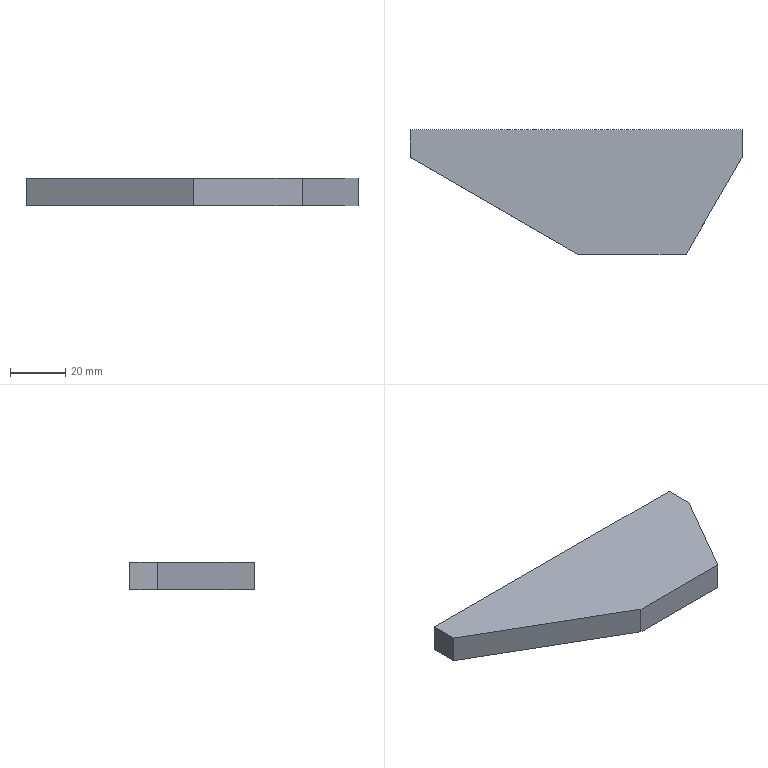Part | SolidWorks | features Extrusion 1 | 1 solid | 8 faces | box 120 x 45 x 10 mm | volume 39855 mm3 | plane 8
STEP:
#1=CARTESIAN_POINT('',(0.,0.,0.));
#2=VERTEX_POINT('',#1);
#3=CARTESIAN_POINT('',(0.,-10.,0.));
#4=VERTEX_POINT('',#3);
#5=CARTESIAN_POINT('',(0.,0.,0.));
#6=DIRECTION('',(0.,-1.,0.));
#7=VECTOR('',#6,1000.);
#8=LINE('',#5,#7);
#9=EDGE_CURVE('',#2,#4,#8,.T.);
#10=ORIENTED_EDGE('',*,*,#9,.T.);
#11=CARTESIAN_POINT('',(0.,-10.,10.));
#12=VERTEX_POINT('',#11);
#13=CARTESIAN_POINT('',(0.,-10.,10.));
#14=DIRECTION('',(0.,0.,-1.));
#15=VECTOR('',#14,1000.);
#16=LINE('',#13,#15);
#17=EDGE_CURVE('',#12,#4,#16,.T.);
#18=ORIENTED_EDGE('',*,*,#17,.F.);
#19=CARTESIAN_POINT('',(0.,0.,10.));
#20=VERTEX_POINT('',#19);
#21=CARTESIAN_POINT('',(0.,0.,10.));
#22=DIRECTION('',(0.,-1.,0.));
#23=VECTOR('',#22,1000.);
#24=LINE('',#21,#23);
#25=EDGE_CURVE('',#20,#12,#24,.T.);
#26=ORIENTED_EDGE('',*,*,#25,.F.);
#27=CARTESIAN_POINT('',(0.,0.,10.));
#28=DIRECTION('',(0.,0.,-1.));
#29=VECTOR('',#28,1000.);
#30=LINE('',#27,#29);
#31=EDGE_CURVE('',#20,#2,#30,.T.);
#32=ORIENTED_EDGE('',*,*,#31,.T.);
#33=EDGE_LOOP('',(#10,#18,#26,#32));
#34=FACE_OUTER_BOUND('',#33,.T.);
#35=CARTESIAN_POINT('',(0.,0.,10.));
#36=DIRECTION('',(1.,0.,0.));
#37=DIRECTION('',(0.,0.,-1.));
#38=AXIS2_PLACEMENT_3D('',#35,#36,#37);
#39=PLANE('',#38);
#40=ADVANCED_FACE('',(#34),#39,.F.);
#41=CARTESIAN_POINT('',(60.622,-45.,0.));
#42=VERTEX_POINT('',#41);
#43=CARTESIAN_POINT('',(60.622,-45.,0.));
#44=DIRECTION('',(0.866,-0.5,0.));
#45=VECTOR('',#44,1000.);
#46=LINE('',#43,#45);
#47=EDGE_CURVE('',#4,#42,#46,.T.);
#48=ORIENTED_EDGE('',*,*,#47,.T.);
#49=CARTESIAN_POINT('',(60.622,-45.,10.));
#50=VERTEX_POINT('',#49);
#51=CARTESIAN_POINT('',(60.622,-45.,10.));
#52=DIRECTION('',(0.,0.,-1.));
#53=VECTOR('',#52,1000.);
#54=LINE('',#51,#53);
#55=EDGE_CURVE('',#50,#42,#54,.T.);
#56=ORIENTED_EDGE('',*,*,#55,.F.);
#57=CARTESIAN_POINT('',(60.622,-45.,10.));
#58=DIRECTION('',(0.866,-0.5,0.));
#59=VECTOR('',#58,1000.);
#60=LINE('',#57,#59);
#61=EDGE_CURVE('',#12,#50,#60,.T.);
#62=ORIENTED_EDGE('',*,*,#61,.F.);
#63=ORIENTED_EDGE('',*,*,#17,.T.);
#64=EDGE_LOOP('',(#48,#56,#62,#63));
#65=FACE_OUTER_BOUND('',#64,.T.);
#66=CARTESIAN_POINT('',(60.622,-45.,10.));
#67=DIRECTION('',(0.5,0.866,0.));
#68=DIRECTION('',(-0.866,0.5,0.));
#69=AXIS2_PLACEMENT_3D('',#66,#67,#68);
#70=PLANE('',#69);
#71=ADVANCED_FACE('',(#65),#70,.F.);
#72=CARTESIAN_POINT('',(99.793,-45.,0.));
#73=VERTEX_POINT('',#72);
#74=CARTESIAN_POINT('',(99.793,-45.,0.));
#75=DIRECTION('',(1.,0.,0.));
#76=VECTOR('',#75,1000.);
#77=LINE('',#74,#76);
#78=EDGE_CURVE('',#42,#73,#77,.T.);
#79=ORIENTED_EDGE('',*,*,#78,.T.);
#80=CARTESIAN_POINT('',(99.793,-45.,10.));
#81=VERTEX_POINT('',#80);
#82=CARTESIAN_POINT('',(99.793,-45.,10.));
#83=DIRECTION('',(0.,0.,-1.));
#84=VECTOR('',#83,1000.);
#85=LINE('',#82,#84);
#86=EDGE_CURVE('',#81,#73,#85,.T.);
#87=ORIENTED_EDGE('',*,*,#86,.F.);
#88=CARTESIAN_POINT('',(99.793,-45.,10.));
#89=DIRECTION('',(1.,0.,0.));
#90=VECTOR('',#89,1000.);
#91=LINE('',#88,#90);
#92=EDGE_CURVE('',#50,#81,#91,.T.);
#93=ORIENTED_EDGE('',*,*,#92,.F.);
#94=ORIENTED_EDGE('',*,*,#55,.T.);
#95=EDGE_LOOP('',(#79,#87,#93,#94));
#96=FACE_OUTER_BOUND('',#95,.T.);
#97=CARTESIAN_POINT('',(99.793,-45.,10.));
#98=DIRECTION('',(0.,1.,0.));
#99=DIRECTION('',(-1.,0.,0.));
#100=AXIS2_PLACEMENT_3D('',#97,#98,#99);
#101=PLANE('',#100);
#102=ADVANCED_FACE('',(#96),#101,.F.);
#103=CARTESIAN_POINT('',(120.,-10.,0.));
#104=VERTEX_POINT('',#103);
#105=CARTESIAN_POINT('',(120.,-10.,0.));
#106=DIRECTION('',(0.5,0.866,0.));
#107=VECTOR('',#106,1000.);
#108=LINE('',#105,#107);
#109=EDGE_CURVE('',#73,#104,#108,.T.);
#110=ORIENTED_EDGE('',*,*,#109,.T.);
#111=CARTESIAN_POINT('',(120.,-10.,10.));
#112=VERTEX_POINT('',#111);
#113=CARTESIAN_POINT('',(120.,-10.,10.));
#114=DIRECTION('',(0.,0.,-1.));
#115=VECTOR('',#114,1000.);
#116=LINE('',#113,#115);
#117=EDGE_CURVE('',#112,#104,#116,.T.);
#118=ORIENTED_EDGE('',*,*,#117,.F.);
#119=CARTESIAN_POINT('',(120.,-10.,10.));
#120=DIRECTION('',(0.5,0.866,0.));
#121=VECTOR('',#120,1000.);
#122=LINE('',#119,#121);
#123=EDGE_CURVE('',#81,#112,#122,.T.);
#124=ORIENTED_EDGE('',*,*,#123,.F.);
#125=ORIENTED_EDGE('',*,*,#86,.T.);
#126=EDGE_LOOP('',(#110,#118,#124,#125));
#127=FACE_OUTER_BOUND('',#126,.T.);
#128=CARTESIAN_POINT('',(120.,-10.,10.));
#129=DIRECTION('',(-0.866,0.5,0.));
#130=DIRECTION('',(-0.5,-0.866,0.));
#131=AXIS2_PLACEMENT_3D('',#128,#129,#130);
#132=PLANE('',#131);
#133=ADVANCED_FACE('',(#127),#132,.F.);
#134=CARTESIAN_POINT('',(120.,0.,0.));
#135=VERTEX_POINT('',#134);
#136=CARTESIAN_POINT('',(120.,0.,0.));
#137=DIRECTION('',(0.,1.,0.));
#138=VECTOR('',#137,1000.);
#139=LINE('',#136,#138);
#140=EDGE_CURVE('',#104,#135,#139,.T.);
#141=ORIENTED_EDGE('',*,*,#140,.T.);
#142=CARTESIAN_POINT('',(120.,0.,10.));
#143=VERTEX_POINT('',#142);
#144=CARTESIAN_POINT('',(120.,0.,10.));
#145=DIRECTION('',(0.,0.,-1.));
#146=VECTOR('',#145,1000.);
#147=LINE('',#144,#146);
#148=EDGE_CURVE('',#143,#135,#147,.T.);
#149=ORIENTED_EDGE('',*,*,#148,.F.);
#150=CARTESIAN_POINT('',(120.,0.,10.));
#151=DIRECTION('',(0.,1.,0.));
#152=VECTOR('',#151,1000.);
#153=LINE('',#150,#152);
#154=EDGE_CURVE('',#112,#143,#153,.T.);
#155=ORIENTED_EDGE('',*,*,#154,.F.);
#156=ORIENTED_EDGE('',*,*,#117,.T.);
#157=EDGE_LOOP('',(#141,#149,#155,#156));
#158=FACE_OUTER_BOUND('',#157,.T.);
#159=CARTESIAN_POINT('',(120.,0.,10.));
#160=DIRECTION('',(-1.,0.,0.));
#161=DIRECTION('',(0.,0.,1.));
#162=AXIS2_PLACEMENT_3D('',#159,#160,#161);
#163=PLANE('',#162);
#164=ADVANCED_FACE('',(#158),#163,.F.);
#165=CARTESIAN_POINT('',(0.,0.,0.));
#166=DIRECTION('',(-1.,0.,0.));
#167=VECTOR('',#166,1000.);
#168=LINE('',#165,#167);
#169=EDGE_CURVE('',#135,#2,#168,.T.);
#170=ORIENTED_EDGE('',*,*,#169,.T.);
#171=ORIENTED_EDGE('',*,*,#31,.F.);
#172=CARTESIAN_POINT('',(0.,0.,10.));
#173=DIRECTION('',(-1.,0.,0.));
#174=VECTOR('',#173,1000.);
#175=LINE('',#172,#174);
#176=EDGE_CURVE('',#143,#20,#175,.T.);
#177=ORIENTED_EDGE('',*,*,#176,.F.);
#178=ORIENTED_EDGE('',*,*,#148,.T.);
#179=EDGE_LOOP('',(#170,#171,#177,#178));
#180=FACE_OUTER_BOUND('',#179,.T.);
#181=CARTESIAN_POINT('',(0.,0.,10.));
#182=DIRECTION('',(0.,-1.,0.));
#183=DIRECTION('',(0.,0.,-1.));
#184=AXIS2_PLACEMENT_3D('',#181,#182,#183);
#185=PLANE('',#184);
#186=ADVANCED_FACE('',(#180),#185,.F.);
#187=ORIENTED_EDGE('',*,*,#25,.T.);
#188=ORIENTED_EDGE('',*,*,#61,.T.);
#189=ORIENTED_EDGE('',*,*,#92,.T.);
#190=ORIENTED_EDGE('',*,*,#123,.T.);
#191=ORIENTED_EDGE('',*,*,#154,.T.);
#192=ORIENTED_EDGE('',*,*,#176,.T.);
#193=EDGE_LOOP('',(#187,#188,#189,#190,#191,#192));
#194=FACE_OUTER_BOUND('',#193,.T.);
#195=CARTESIAN_POINT('',(0.,0.,10.));
#196=DIRECTION('',(0.,0.,-1.));
#197=DIRECTION('',(-1.,0.,0.));
#198=AXIS2_PLACEMENT_3D('',#195,#196,#197);
#199=PLANE('',#198);
#200=ADVANCED_FACE('',(#194),#199,.F.);
#201=ORIENTED_EDGE('',*,*,#9,.F.);
#202=ORIENTED_EDGE('',*,*,#169,.F.);
#203=ORIENTED_EDGE('',*,*,#140,.F.);
#204=ORIENTED_EDGE('',*,*,#109,.F.);
#205=ORIENTED_EDGE('',*,*,#78,.F.);
#206=ORIENTED_EDGE('',*,*,#47,.F.);
#207=EDGE_LOOP('',(#201,#202,#203,#204,#205,#206));
#208=FACE_OUTER_BOUND('',#207,.T.);
#209=CARTESIAN_POINT('',(0.,0.,0.));
#210=DIRECTION('',(0.,0.,-1.));
#211=DIRECTION('',(-1.,0.,0.));
#212=AXIS2_PLACEMENT_3D('',#209,#210,#211);
#213=PLANE('',#212);
#214=ADVANCED_FACE('',(#208),#213,.T.);
#215=CLOSED_SHELL('',(#40,#71,#102,#133,#164,#186,#200,#214));
#216=MANIFOLD_SOLID_BREP('',#215);
#217=CARTESIAN_POINT('',(0.,0.,0.));
#218=DIRECTION('',(0.,0.,1.));
#219=DIRECTION('',(1.,0.,0.));
#220=AXIS2_PLACEMENT_3D('',#217,#218,#219);
#221=(LENGTH_UNIT()NAMED_UNIT(*)SI_UNIT(.MILLI.,.METRE.));
#222=UNCERTAINTY_MEASURE_WITH_UNIT(LENGTH_MEASURE(0.00001),#221,'','');
#223=(NAMED_UNIT(*)PLANE_ANGLE_UNIT()SI_UNIT($,.RADIAN.));
#224=(NAMED_UNIT(*)SI_UNIT($,.STERADIAN.)SOLID_ANGLE_UNIT());
#225=(GEOMETRIC_REPRESENTATION_CONTEXT(3)GLOBAL_UNCERTAINTY_ASSIGNED_CONTEXT((#222))GLOBAL_UNIT_ASSIGNED_CONTEXT((#221,#223,#224))REPRESENTATION_CONTEXT('',''));
#226=ADVANCED_BREP_SHAPE_REPRESENTATION('',(#216,#220),#225);